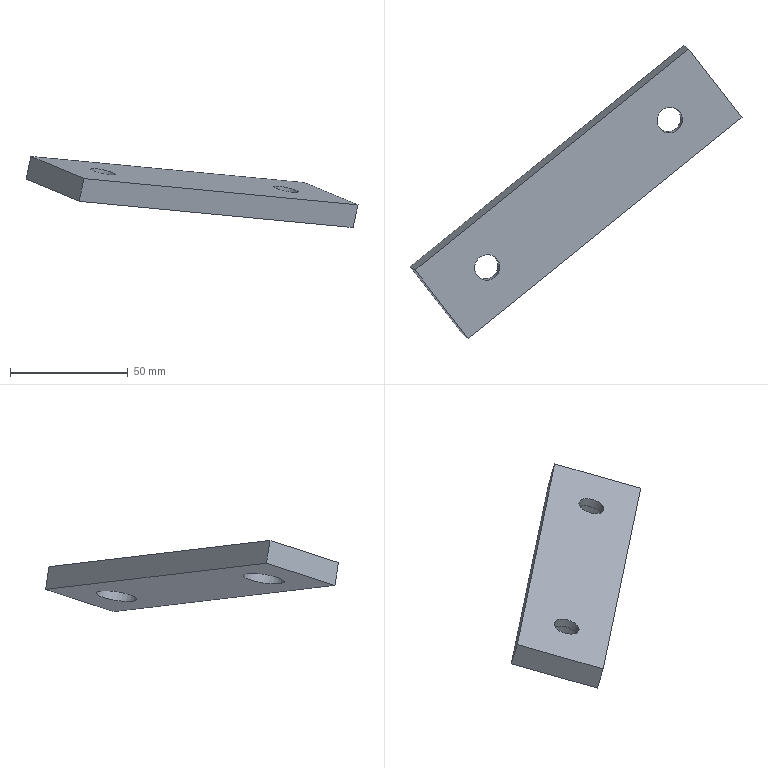Part | NX | features solid 2 | 1 solid | 12 faces | box 141.116 x 124.485 x 30.205 mm | volume 53266 mm3 | plane 8 | cylinder 4 | commonest cylinder face diameters 11 x2 17.5 x2
STEP:
#1=CARTESIAN_POINT('',(-418.352,533.293,89.12));
#2=VERTEX_POINT('',#1);
#3=CARTESIAN_POINT('',(-395.79,504.204,79.697));
#4=VERTEX_POINT('',#3);
#5=CARTESIAN_POINT('',(-418.352,533.293,89.12));
#6=DIRECTION('',(0.5937,-0.7655,-0.248));
#7=VECTOR('',#6,1000.);
#8=LINE('',#5,#7);
#9=EDGE_CURVE('',#2,#4,#8,.T.);
#10=ORIENTED_EDGE('',*,*,#9,.F.);
#11=CARTESIAN_POINT('',(-420.472,534.778,79.461));
#12=VERTEX_POINT('',#11);
#13=CARTESIAN_POINT('',(-420.472,534.778,79.461));
#14=DIRECTION('',(0.212,-0.1485,0.9659));
#15=VECTOR('',#14,1000.);
#16=LINE('',#13,#15);
#17=EDGE_CURVE('',#12,#2,#16,.T.);
#18=ORIENTED_EDGE('',*,*,#17,.F.);
#19=CARTESIAN_POINT('',(-397.91,505.689,70.038));
#20=VERTEX_POINT('',#19);
#21=CARTESIAN_POINT('',(-420.472,534.778,79.461));
#22=DIRECTION('',(0.5937,-0.7655,-0.248));
#23=VECTOR('',#22,1000.);
#24=LINE('',#21,#23);
#25=EDGE_CURVE('',#12,#20,#24,.T.);
#26=ORIENTED_EDGE('',*,*,#25,.T.);
#27=CARTESIAN_POINT('',(-397.91,505.689,70.038));
#28=DIRECTION('',(0.212,-0.1485,0.9659));
#29=VECTOR('',#28,1000.);
#30=LINE('',#27,#29);
#31=EDGE_CURVE('',#20,#4,#30,.T.);
#32=ORIENTED_EDGE('',*,*,#31,.T.);
#33=EDGE_LOOP('',(#10,#18,#26,#32));
#34=FACE_BOUND('',#33,.T.);
#35=CARTESIAN_POINT('',(-420.472,534.778,79.461));
#36=DIRECTION('',(-0.7762,-0.6261,0.07415));
#37=DIRECTION('',(0.6278,-0.7784,0.));
#38=AXIS2_PLACEMENT_3D('',#35,#36,#37);
#39=PLANE('',#38);
#40=ADVANCED_FACE('',(#34),#39,.T.);
#41=CARTESIAN_POINT('',(-279.356,598.115,68.574));
#42=VERTEX_POINT('',#41);
#43=CARTESIAN_POINT('',(-279.356,598.115,68.574));
#44=DIRECTION('',(-0.7762,-0.6261,0.07415));
#45=VECTOR('',#44,1000.);
#46=LINE('',#43,#45);
#47=EDGE_CURVE('',#42,#4,#46,.T.);
#48=ORIENTED_EDGE('',*,*,#47,.T.);
#49=ORIENTED_EDGE('',*,*,#31,.F.);
#50=CARTESIAN_POINT('',(-281.476,599.6,58.915));
#51=VERTEX_POINT('',#50);
#52=CARTESIAN_POINT('',(-281.476,599.6,58.915));
#53=DIRECTION('',(-0.7762,-0.6261,0.07415));
#54=VECTOR('',#53,1000.);
#55=LINE('',#52,#54);
#56=EDGE_CURVE('',#51,#20,#55,.T.);
#57=ORIENTED_EDGE('',*,*,#56,.F.);
#58=CARTESIAN_POINT('',(-281.476,599.6,58.915));
#59=DIRECTION('',(0.212,-0.1485,0.9659));
#60=VECTOR('',#59,1000.);
#61=LINE('',#58,#60);
#62=EDGE_CURVE('',#51,#42,#61,.T.);
#63=ORIENTED_EDGE('',*,*,#62,.T.);
#64=EDGE_LOOP('',(#48,#49,#57,#63));
#65=FACE_BOUND('',#64,.T.);
#66=CARTESIAN_POINT('',(-281.476,599.6,58.915));
#67=DIRECTION('',(-0.5937,0.7655,0.248));
#68=DIRECTION('',(-0.7902,-0.6129,0.));
#69=AXIS2_PLACEMENT_3D('',#66,#67,#68);
#70=PLANE('',#69);
#71=ADVANCED_FACE('',(#65),#70,.F.);
#72=CARTESIAN_POINT('',(-301.918,627.204,77.997));
#73=VERTEX_POINT('',#72);
#74=CARTESIAN_POINT('',(-301.918,627.204,77.997));
#75=DIRECTION('',(0.5937,-0.7655,-0.248));
#76=VECTOR('',#75,1000.);
#77=LINE('',#74,#76);
#78=EDGE_CURVE('',#73,#42,#77,.T.);
#79=ORIENTED_EDGE('',*,*,#78,.T.);
#80=ORIENTED_EDGE('',*,*,#62,.F.);
#81=CARTESIAN_POINT('',(-304.038,628.689,68.338));
#82=VERTEX_POINT('',#81);
#83=CARTESIAN_POINT('',(-304.038,628.689,68.338));
#84=DIRECTION('',(0.5937,-0.7655,-0.248));
#85=VECTOR('',#84,1000.);
#86=LINE('',#83,#85);
#87=EDGE_CURVE('',#82,#51,#86,.T.);
#88=ORIENTED_EDGE('',*,*,#87,.F.);
#89=CARTESIAN_POINT('',(-304.038,628.689,68.338));
#90=DIRECTION('',(0.212,-0.1485,0.9659));
#91=VECTOR('',#90,1000.);
#92=LINE('',#89,#91);
#93=EDGE_CURVE('',#82,#73,#92,.T.);
#94=ORIENTED_EDGE('',*,*,#93,.T.);
#95=EDGE_LOOP('',(#79,#80,#88,#94));
#96=FACE_BOUND('',#95,.T.);
#97=CARTESIAN_POINT('',(-304.038,628.689,68.338));
#98=DIRECTION('',(-0.7762,-0.6261,0.07415));
#99=DIRECTION('',(0.6278,-0.7784,0.));
#100=AXIS2_PLACEMENT_3D('',#97,#98,#99);
#101=PLANE('',#100);
#102=ADVANCED_FACE('',(#96),#101,.F.);
#103=CARTESIAN_POINT('',(-418.352,533.293,89.12));
#104=DIRECTION('',(0.7762,0.6261,-0.07415));
#105=VECTOR('',#104,1000.);
#106=LINE('',#103,#105);
#107=EDGE_CURVE('',#2,#73,#106,.T.);
#108=ORIENTED_EDGE('',*,*,#107,.T.);
#109=ORIENTED_EDGE('',*,*,#93,.F.);
#110=CARTESIAN_POINT('',(-420.472,534.778,79.461));
#111=DIRECTION('',(0.7762,0.6261,-0.07415));
#112=VECTOR('',#111,1000.);
#113=LINE('',#110,#112);
#114=EDGE_CURVE('',#12,#82,#113,.T.);
#115=ORIENTED_EDGE('',*,*,#114,.F.);
#116=ORIENTED_EDGE('',*,*,#17,.T.);
#117=EDGE_LOOP('',(#108,#109,#115,#116));
#118=FACE_BOUND('',#117,.T.);
#119=CARTESIAN_POINT('',(-420.472,534.778,79.461));
#120=DIRECTION('',(0.5937,-0.7655,-0.248));
#121=DIRECTION('',(0.7902,0.6129,0.));
#122=AXIS2_PLACEMENT_3D('',#119,#120,#121);
#123=PLANE('',#122);
#124=ADVANCED_FACE('',(#118),#123,.F.);
#125=CARTESIAN_POINT('',(-381.239,535.885,71.02));
#126=VERTEX_POINT('',#125);
#127=CARTESIAN_POINT('',(-389.786,535.885,72.896));
#128=DIRECTION('',(0.212,-0.1485,0.9659));
#129=DIRECTION('',(0.9767,0.,-0.2144));
#130=AXIS2_PLACEMENT_3D('',#127,#128,#129);
#131=CIRCLE('',#130,8.75);
#132=EDGE_CURVE('',#126,#126,#131,.T.);
#133=ORIENTED_EDGE('',*,*,#132,.T.);
#134=EDGE_LOOP('',(#133));
#135=FACE_BOUND('',#134,.T.);
#136=CARTESIAN_POINT('',(-303.616,598.492,63.604));
#137=VERTEX_POINT('',#136);
#138=CARTESIAN_POINT('',(-312.163,598.492,65.48));
#139=DIRECTION('',(0.212,-0.1485,0.9659));
#140=DIRECTION('',(0.9767,0.,-0.2144));
#141=AXIS2_PLACEMENT_3D('',#138,#139,#140);
#142=CIRCLE('',#141,8.75);
#143=EDGE_CURVE('',#137,#137,#142,.T.);
#144=ORIENTED_EDGE('',*,*,#143,.T.);
#145=EDGE_LOOP('',(#144));
#146=FACE_BOUND('',#145,.T.);
#147=ORIENTED_EDGE('',*,*,#25,.F.);
#148=ORIENTED_EDGE('',*,*,#114,.T.);
#149=ORIENTED_EDGE('',*,*,#87,.T.);
#150=ORIENTED_EDGE('',*,*,#56,.T.);
#151=EDGE_LOOP('',(#147,#148,#149,#150));
#152=FACE_BOUND('',#151,.T.);
#153=CARTESIAN_POINT('',(285.974,581.689,-68.388));
#154=DIRECTION('',(-0.212,0.1485,-0.9659));
#155=DIRECTION('',(-0.9767,0.,0.2144));
#156=AXIS2_PLACEMENT_3D('',#153,#154,#155);
#157=PLANE('',#156);
#158=ADVANCED_FACE('',(#135,#146,#152),#157,.T.);
#159=CARTESIAN_POINT('',(-393.038,534.4,83.734));
#160=VERTEX_POINT('',#159);
#161=CARTESIAN_POINT('',(-387.666,534.4,82.555));
#162=DIRECTION('',(-0.212,0.1485,-0.9659));
#163=DIRECTION('',(-0.9767,0.,0.2144));
#164=AXIS2_PLACEMENT_3D('',#161,#162,#163);
#165=CIRCLE('',#164,5.5);
#166=EDGE_CURVE('',#160,#160,#165,.T.);
#167=ORIENTED_EDGE('',*,*,#166,.T.);
#168=EDGE_LOOP('',(#167));
#169=FACE_BOUND('',#168,.T.);
#170=CARTESIAN_POINT('',(-315.415,597.008,76.319));
#171=VERTEX_POINT('',#170);
#172=CARTESIAN_POINT('',(-310.043,597.008,75.139));
#173=DIRECTION('',(-0.212,0.1485,-0.9659));
#174=DIRECTION('',(-0.9767,0.,0.2144));
#175=AXIS2_PLACEMENT_3D('',#172,#173,#174);
#176=CIRCLE('',#175,5.5);
#177=EDGE_CURVE('',#171,#171,#176,.T.);
#178=ORIENTED_EDGE('',*,*,#177,.T.);
#179=EDGE_LOOP('',(#178));
#180=FACE_BOUND('',#179,.T.);
#181=ORIENTED_EDGE('',*,*,#9,.T.);
#182=ORIENTED_EDGE('',*,*,#47,.F.);
#183=ORIENTED_EDGE('',*,*,#78,.F.);
#184=ORIENTED_EDGE('',*,*,#107,.F.);
#185=EDGE_LOOP('',(#181,#182,#183,#184));
#186=FACE_BOUND('',#185,.T.);
#187=CARTESIAN_POINT('',(288.094,580.205,-58.729));
#188=DIRECTION('',(-0.212,0.1485,-0.9659));
#189=DIRECTION('',(-0.9767,0.,0.2144));
#190=AXIS2_PLACEMENT_3D('',#187,#188,#189);
#191=PLANE('',#190);
#192=ADVANCED_FACE('',(#169,#180,#186),#191,.F.);
#193=CARTESIAN_POINT('',(-305.455,597.557,70.386));
#194=VERTEX_POINT('',#193);
#195=CARTESIAN_POINT('',(-310.827,597.557,71.565));
#196=DIRECTION('',(0.212,-0.1485,0.9659));
#197=DIRECTION('',(0.9767,0.,-0.2144));
#198=AXIS2_PLACEMENT_3D('',#195,#196,#197);
#199=CIRCLE('',#198,5.5);
#200=EDGE_CURVE('',#194,#194,#199,.T.);
#201=ORIENTED_EDGE('',*,*,#200,.F.);
#202=EDGE_LOOP('',(#201));
#203=FACE_BOUND('',#202,.T.);
#204=ORIENTED_EDGE('',*,*,#177,.F.);
#205=EDGE_LOOP('',(#204));
#206=FACE_BOUND('',#205,.T.);
#207=CARTESIAN_POINT('',(-301.562,591.07,113.776));
#208=DIRECTION('',(0.212,-0.1485,0.9659));
#209=DIRECTION('',(0.9767,0.,-0.2144));
#210=AXIS2_PLACEMENT_3D('',#207,#208,#209);
#211=CYLINDRICAL_SURFACE('',#210,5.5);
#212=ADVANCED_FACE('',(#203,#206),#211,.F.);
#213=ORIENTED_EDGE('',*,*,#200,.T.);
#214=EDGE_LOOP('',(#213));
#215=FACE_BOUND('',#214,.T.);
#216=CARTESIAN_POINT('',(-302.28,597.557,69.69));
#217=VERTEX_POINT('',#216);
#218=CARTESIAN_POINT('',(-310.827,597.557,71.565));
#219=DIRECTION('',(0.212,-0.1485,0.9659));
#220=DIRECTION('',(0.9767,0.,-0.2144));
#221=AXIS2_PLACEMENT_3D('',#218,#219,#220);
#222=CIRCLE('',#221,8.75);
#223=EDGE_CURVE('',#217,#217,#222,.T.);
#224=ORIENTED_EDGE('',*,*,#223,.F.);
#225=EDGE_LOOP('',(#224));
#226=FACE_BOUND('',#225,.T.);
#227=CARTESIAN_POINT('',(-310.827,597.557,71.565));
#228=DIRECTION('',(0.212,-0.1485,0.9659));
#229=DIRECTION('',(0.9767,0.,-0.2144));
#230=AXIS2_PLACEMENT_3D('',#227,#228,#229);
#231=PLANE('',#230);
#232=ADVANCED_FACE('',(#215,#226),#231,.F.);
#233=ORIENTED_EDGE('',*,*,#223,.T.);
#234=EDGE_LOOP('',(#233));
#235=FACE_BOUND('',#234,.T.);
#236=ORIENTED_EDGE('',*,*,#143,.F.);
#237=EDGE_LOOP('',(#236));
#238=FACE_BOUND('',#237,.T.);
#239=CARTESIAN_POINT('',(-312.163,598.492,65.48));
#240=DIRECTION('',(0.212,-0.1485,0.9659));
#241=DIRECTION('',(0.9767,0.,-0.2144));
#242=AXIS2_PLACEMENT_3D('',#239,#240,#241);
#243=CYLINDRICAL_SURFACE('',#242,8.75);
#244=ADVANCED_FACE('',(#235,#238),#243,.F.);
#245=CARTESIAN_POINT('',(-383.078,534.95,77.802));
#246=VERTEX_POINT('',#245);
#247=CARTESIAN_POINT('',(-388.45,534.95,78.981));
#248=DIRECTION('',(0.212,-0.1485,0.9659));
#249=DIRECTION('',(0.9767,0.,-0.2144));
#250=AXIS2_PLACEMENT_3D('',#247,#248,#249);
#251=CIRCLE('',#250,5.5);
#252=EDGE_CURVE('',#246,#246,#251,.T.);
#253=ORIENTED_EDGE('',*,*,#252,.F.);
#254=EDGE_LOOP('',(#253));
#255=FACE_BOUND('',#254,.T.);
#256=ORIENTED_EDGE('',*,*,#166,.F.);
#257=EDGE_LOOP('',(#256));
#258=FACE_BOUND('',#257,.T.);
#259=CARTESIAN_POINT('',(-379.185,528.462,121.192));
#260=DIRECTION('',(0.212,-0.1485,0.9659));
#261=DIRECTION('',(0.9767,0.,-0.2144));
#262=AXIS2_PLACEMENT_3D('',#259,#260,#261);
#263=CYLINDRICAL_SURFACE('',#262,5.5);
#264=ADVANCED_FACE('',(#255,#258),#263,.F.);
#265=ORIENTED_EDGE('',*,*,#252,.T.);
#266=EDGE_LOOP('',(#265));
#267=FACE_BOUND('',#266,.T.);
#268=CARTESIAN_POINT('',(-379.903,534.95,77.105));
#269=VERTEX_POINT('',#268);
#270=CARTESIAN_POINT('',(-388.45,534.95,78.981));
#271=DIRECTION('',(0.212,-0.1485,0.9659));
#272=DIRECTION('',(0.9767,0.,-0.2144));
#273=AXIS2_PLACEMENT_3D('',#270,#271,#272);
#274=CIRCLE('',#273,8.75);
#275=EDGE_CURVE('',#269,#269,#274,.T.);
#276=ORIENTED_EDGE('',*,*,#275,.F.);
#277=EDGE_LOOP('',(#276));
#278=FACE_BOUND('',#277,.T.);
#279=CARTESIAN_POINT('',(-388.45,534.95,78.981));
#280=DIRECTION('',(0.212,-0.1485,0.9659));
#281=DIRECTION('',(0.9767,0.,-0.2144));
#282=AXIS2_PLACEMENT_3D('',#279,#280,#281);
#283=PLANE('',#282);
#284=ADVANCED_FACE('',(#267,#278),#283,.F.);
#285=ORIENTED_EDGE('',*,*,#275,.T.);
#286=EDGE_LOOP('',(#285));
#287=FACE_BOUND('',#286,.T.);
#288=ORIENTED_EDGE('',*,*,#132,.F.);
#289=EDGE_LOOP('',(#288));
#290=FACE_BOUND('',#289,.T.);
#291=CARTESIAN_POINT('',(-389.786,535.885,72.896));
#292=DIRECTION('',(0.212,-0.1485,0.9659));
#293=DIRECTION('',(0.9767,0.,-0.2144));
#294=AXIS2_PLACEMENT_3D('',#291,#292,#293);
#295=CYLINDRICAL_SURFACE('',#294,8.75);
#296=ADVANCED_FACE('',(#287,#290),#295,.F.);
#297=CLOSED_SHELL('',(#40,#71,#102,#124,#158,#192,#212,#232,#244,#264,#284,#296));
#298=MANIFOLD_SOLID_BREP('',#297);
#299=(LENGTH_UNIT()NAMED_UNIT(*)SI_UNIT(.MILLI.,.METRE.));
#300=UNCERTAINTY_MEASURE_WITH_UNIT(LENGTH_MEASURE(0.00001),#299,'','');
#301=(NAMED_UNIT(*)PLANE_ANGLE_UNIT()SI_UNIT($,.RADIAN.));
#302=(NAMED_UNIT(*)SI_UNIT($,.STERADIAN.)SOLID_ANGLE_UNIT());
#303=(GEOMETRIC_REPRESENTATION_CONTEXT(3)GLOBAL_UNCERTAINTY_ASSIGNED_CONTEXT((#300))GLOBAL_UNIT_ASSIGNED_CONTEXT((#299,#301,#302))REPRESENTATION_CONTEXT('',''));
#304=ADVANCED_BREP_SHAPE_REPRESENTATION('',(#298),#303);